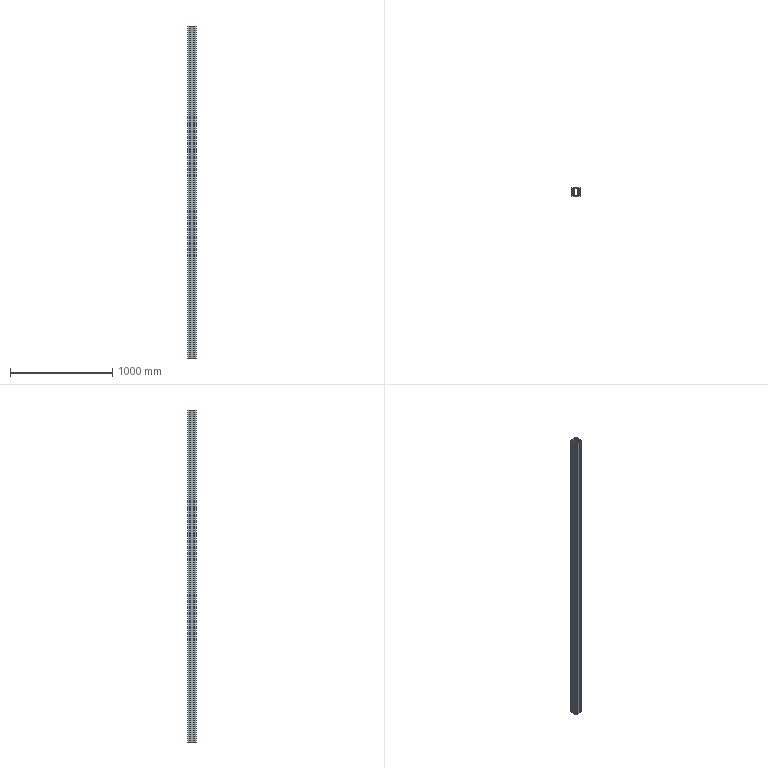Part | NX | features BREP 1 | 1 solid | 130 faces | box 80 x 80 x 3250 mm | volume 7997163 mm3 | plane 114 | cylinder 16 | commonest cylinder face diameters 6.8 x16